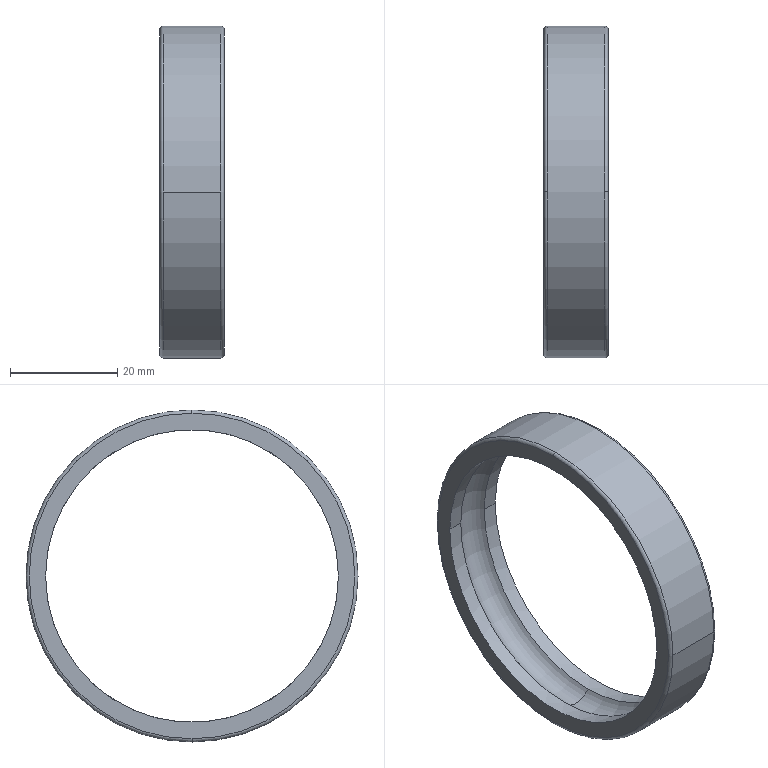Part | STEP file | bearing_6908_02V11 | 1 solid | 14 faces | box 12 x 62 x 62 mm | volume 6668 mm3 | cylinder 6 | torus 6 | plane 2 | commonest cylinder face diameters 54.67 x4 62 x2
STEP:
#1=CARTESIAN_POINT('',(0.,0.,0.));
#2=DIRECTION('',(0.,0.,1.));
#3=DIRECTION('',(1.,0.,0.));
#4=AXIS2_PLACEMENT_3D('',#1,#2,#3);
#5=CARTESIAN_POINT('',(-3.096,27.335,0.));
#6=VERTEX_POINT('',#5);
#7=CARTESIAN_POINT('',(-3.096,0.,27.335));
#8=VERTEX_POINT('',#7);
#9=CARTESIAN_POINT('',(-3.096,0.,0.));
#10=DIRECTION('',(1.,0.,0.));
#11=DIRECTION('',(0.,1.,0.));
#12=AXIS2_PLACEMENT_3D('',#9,#10,#11);
#13=CIRCLE('',#12,27.335);
#14=CARTESIAN_POINT('',(-4.548,0.,0.));
#15=DIRECTION('',(-1.,0.,0.));
#16=DIRECTION('',(0.,1.,0.));
#17=AXIS2_PLACEMENT_3D('',#14,#15,#16);
#18=CYLINDRICAL_SURFACE('',#17,27.335);
#19=CARTESIAN_POINT('',(6.283,-1.452));
#20=DIRECTION('',(-1.,0.));
#21=VECTOR('',#20,1.);
#22=LINE('',#19,#21);
#23=(GEOMETRIC_REPRESENTATION_CONTEXT(2)PARAMETRIC_REPRESENTATION_CONTEXT()REPRESENTATION_CONTEXT('',''));
#24=DEFINITIONAL_REPRESENTATION('',(#22),#23);
#25=PCURVE('',#18,#24);
#26=CARTESIAN_POINT('',(0.,0.,0.));
#27=DIRECTION('',(1.,0.,0.));
#28=DIRECTION('',(0.,0.,-1.));
#29=AXIS2_PLACEMENT_3D('',#26,#27,#28);
#30=TOROIDAL_SURFACE('',#29,25.497,3.6);
#31=CARTESIAN_POINT('',(1.571,-1.035));
#32=DIRECTION('',(1.,0.));
#33=VECTOR('',#32,1.);
#34=LINE('',#31,#33);
#35=(GEOMETRIC_REPRESENTATION_CONTEXT(2)PARAMETRIC_REPRESENTATION_CONTEXT()REPRESENTATION_CONTEXT('',''));
#36=DEFINITIONAL_REPRESENTATION('',(#34),#35);
#37=PCURVE('',#30,#36);
#38=SURFACE_CURVE('',#13,(#25,#37),.PCURVE_S1.);
#39=EDGE_CURVE('',#6,#8,#38,.T.);
#40=ORIENTED_EDGE('',*,*,#39,.F.);
#41=CARTESIAN_POINT('',(-6.,27.335,0.));
#42=VERTEX_POINT('',#41);
#43=CARTESIAN_POINT('',(-4.548,27.335,0.));
#44=DIRECTION('',(-1.,0.,0.));
#45=VECTOR('',#44,1.);
#46=LINE('',#43,#45);
#47=CARTESIAN_POINT('',(6.283,0.));
#48=DIRECTION('',(0.,1.));
#49=VECTOR('',#48,1.);
#50=LINE('',#47,#49);
#51=(GEOMETRIC_REPRESENTATION_CONTEXT(2)PARAMETRIC_REPRESENTATION_CONTEXT()REPRESENTATION_CONTEXT('',''));
#52=DEFINITIONAL_REPRESENTATION('',(#50),#51);
#53=PCURVE('',#18,#52);
#54=CARTESIAN_POINT('',(-4.548,0.,0.));
#55=DIRECTION('',(-1.,0.,0.));
#56=DIRECTION('',(0.,1.,0.));
#57=AXIS2_PLACEMENT_3D('',#54,#55,#56);
#58=CYLINDRICAL_SURFACE('',#57,27.335);
#59=CARTESIAN_POINT('',(0.,0.));
#60=DIRECTION('',(0.,1.));
#61=VECTOR('',#60,1.);
#62=LINE('',#59,#61);
#63=(GEOMETRIC_REPRESENTATION_CONTEXT(2)PARAMETRIC_REPRESENTATION_CONTEXT()REPRESENTATION_CONTEXT('',''));
#64=DEFINITIONAL_REPRESENTATION('',(#62),#63);
#65=PCURVE('',#58,#64);
#66=SURFACE_CURVE('',#46,(#53,#65),.PCURVE_S1.);
#67=EDGE_CURVE('',#6,#42,#66,.T.);
#68=ORIENTED_EDGE('',*,*,#67,.T.);
#69=CARTESIAN_POINT('',(-6.,-27.335,0.));
#70=VERTEX_POINT('',#69);
#71=CARTESIAN_POINT('',(-6.,0.,0.));
#72=DIRECTION('',(1.,0.,0.));
#73=DIRECTION('',(0.,1.,0.));
#74=AXIS2_PLACEMENT_3D('',#71,#72,#73);
#75=CIRCLE('',#74,27.335);
#76=CARTESIAN_POINT('',(6.283,1.452));
#77=DIRECTION('',(-1.,0.));
#78=VECTOR('',#77,1.);
#79=LINE('',#76,#78);
#80=(GEOMETRIC_REPRESENTATION_CONTEXT(2)PARAMETRIC_REPRESENTATION_CONTEXT()REPRESENTATION_CONTEXT('',''));
#81=DEFINITIONAL_REPRESENTATION('',(#79),#80);
#82=PCURVE('',#18,#81);
#83=CARTESIAN_POINT('',(-6.,28.867,0.));
#84=DIRECTION('',(-1.,0.,0.));
#85=DIRECTION('',(0.,-1.,0.));
#86=AXIS2_PLACEMENT_3D('',#83,#84,#85);
#87=PLANE('',#86);
#88=CARTESIAN_POINT('',(1.532,0.));
#89=CARTESIAN_POINT('',(1.532,47.346));
#90=CARTESIAN_POINT('',(42.535,23.673));
#91=CARTESIAN_POINT('',(83.537,0.));
#92=CARTESIAN_POINT('',(42.535,-23.673));
#93=CARTESIAN_POINT('',(1.532,-47.346));
#94=CARTESIAN_POINT('',(1.532,0.));
#95=(BOUNDED_CURVE()B_SPLINE_CURVE(2,(#88,#89,#90,#91,#92,#93,#94),.UNSPECIFIED.,.T.,.F.)B_SPLINE_CURVE_WITH_KNOTS((1,2,2,2,2,1),(-2.094,0.,2.094,4.189,6.283,8.378),.UNSPECIFIED.)CURVE()GEOMETRIC_REPRESENTATION_ITEM()RATIONAL_B_SPLINE_CURVE((1.,0.5,1.,0.5,1.,0.5,1.))REPRESENTATION_ITEM(''));
#96=(GEOMETRIC_REPRESENTATION_CONTEXT(2)PARAMETRIC_REPRESENTATION_CONTEXT()REPRESENTATION_CONTEXT('',''));
#97=DEFINITIONAL_REPRESENTATION('',(#95),#96);
#98=PCURVE('',#87,#97);
#99=SURFACE_CURVE('',#75,(#82,#98),.PCURVE_S1.);
#100=EDGE_CURVE('',#42,#70,#99,.T.);
#101=ORIENTED_EDGE('',*,*,#100,.T.);
#102=CARTESIAN_POINT('',(-3.096,-27.335,0.));
#103=VERTEX_POINT('',#102);
#104=CARTESIAN_POINT('',(-4.548,-27.335,0.));
#105=DIRECTION('',(-1.,0.,0.));
#106=VECTOR('',#105,1.);
#107=LINE('',#104,#106);
#108=CARTESIAN_POINT('',(3.142,0.));
#109=DIRECTION('',(0.,1.));
#110=VECTOR('',#109,1.);
#111=LINE('',#108,#110);
#112=(GEOMETRIC_REPRESENTATION_CONTEXT(2)PARAMETRIC_REPRESENTATION_CONTEXT()REPRESENTATION_CONTEXT('',''));
#113=DEFINITIONAL_REPRESENTATION('',(#111),#112);
#114=PCURVE('',#18,#113);
#115=CARTESIAN_POINT('',(3.142,0.));
#116=DIRECTION('',(0.,1.));
#117=VECTOR('',#116,1.);
#118=LINE('',#115,#117);
#119=(GEOMETRIC_REPRESENTATION_CONTEXT(2)PARAMETRIC_REPRESENTATION_CONTEXT()REPRESENTATION_CONTEXT('',''));
#120=DEFINITIONAL_REPRESENTATION('',(#118),#119);
#121=PCURVE('',#58,#120);
#122=SURFACE_CURVE('',#107,(#114,#121),.PCURVE_S1.);
#123=EDGE_CURVE('',#103,#70,#122,.T.);
#124=ORIENTED_EDGE('',*,*,#123,.F.);
#125=CARTESIAN_POINT('',(-3.096,0.,0.));
#126=DIRECTION('',(1.,0.,0.));
#127=DIRECTION('',(0.,1.,0.));
#128=AXIS2_PLACEMENT_3D('',#125,#126,#127);
#129=CIRCLE('',#128,27.335);
#130=CARTESIAN_POINT('',(6.283,-1.452));
#131=DIRECTION('',(-1.,0.));
#132=VECTOR('',#131,1.);
#133=LINE('',#130,#132);
#134=(GEOMETRIC_REPRESENTATION_CONTEXT(2)PARAMETRIC_REPRESENTATION_CONTEXT()REPRESENTATION_CONTEXT('',''));
#135=DEFINITIONAL_REPRESENTATION('',(#133),#134);
#136=PCURVE('',#18,#135);
#137=CARTESIAN_POINT('',(0.,0.,0.));
#138=DIRECTION('',(1.,0.,0.));
#139=DIRECTION('',(0.,0.,-1.));
#140=AXIS2_PLACEMENT_3D('',#137,#138,#139);
#141=TOROIDAL_SURFACE('',#140,25.497,3.6);
#142=CARTESIAN_POINT('',(1.571,5.248));
#143=DIRECTION('',(1.,0.));
#144=VECTOR('',#143,1.);
#145=LINE('',#142,#144);
#146=(GEOMETRIC_REPRESENTATION_CONTEXT(2)PARAMETRIC_REPRESENTATION_CONTEXT()REPRESENTATION_CONTEXT('',''));
#147=DEFINITIONAL_REPRESENTATION('',(#145),#146);
#148=PCURVE('',#141,#147);
#149=SURFACE_CURVE('',#129,(#136,#148),.PCURVE_S1.);
#150=EDGE_CURVE('',#8,#103,#149,.T.);
#151=ORIENTED_EDGE('',*,*,#150,.F.);
#152=EDGE_LOOP('',(#40,#68,#101,#124,#151));
#153=FACE_BOUND('',#152,.F.);
#154=ADVANCED_FACE('',(#153),#18,.F.);
#155=CARTESIAN_POINT('',(-6.,0.,-30.4));
#156=VERTEX_POINT('',#155);
#157=CARTESIAN_POINT('',(-6.,0.,30.4));
#158=VERTEX_POINT('',#157);
#159=CARTESIAN_POINT('',(-6.,0.,0.));
#160=DIRECTION('',(1.,0.,0.));
#161=DIRECTION('',(0.,1.,0.));
#162=AXIS2_PLACEMENT_3D('',#159,#160,#161);
#163=CIRCLE('',#162,30.4);
#164=CARTESIAN_POINT('',(-5.4,0.,0.));
#165=DIRECTION('',(1.,0.,0.));
#166=DIRECTION('',(0.,0.,-1.));
#167=AXIS2_PLACEMENT_3D('',#164,#165,#166);
#168=TOROIDAL_SURFACE('',#167,30.4,0.6);
#169=CARTESIAN_POINT('',(-4.712,4.712));
#170=DIRECTION('',(1.,0.));
#171=VECTOR('',#170,1.);
#172=LINE('',#169,#171);
#173=(GEOMETRIC_REPRESENTATION_CONTEXT(2)PARAMETRIC_REPRESENTATION_CONTEXT()REPRESENTATION_CONTEXT('',''));
#174=DEFINITIONAL_REPRESENTATION('',(#172),#173);
#175=PCURVE('',#168,#174);
#176=CARTESIAN_POINT('',(-1.532,0.));
#177=CARTESIAN_POINT('',(-1.532,52.654));
#178=CARTESIAN_POINT('',(44.068,26.327));
#179=CARTESIAN_POINT('',(89.668,0.));
#180=CARTESIAN_POINT('',(44.068,-26.327));
#181=CARTESIAN_POINT('',(-1.532,-52.654));
#182=CARTESIAN_POINT('',(-1.532,0.));
#183=(BOUNDED_CURVE()B_SPLINE_CURVE(2,(#176,#177,#178,#179,#180,#181,#182),.UNSPECIFIED.,.T.,.F.)B_SPLINE_CURVE_WITH_KNOTS((1,2,2,2,2,1),(-2.094,0.,2.094,4.189,6.283,8.378),.UNSPECIFIED.)CURVE()GEOMETRIC_REPRESENTATION_ITEM()RATIONAL_B_SPLINE_CURVE((1.,0.5,1.,0.5,1.,0.5,1.))REPRESENTATION_ITEM(''));
#184=(GEOMETRIC_REPRESENTATION_CONTEXT(2)PARAMETRIC_REPRESENTATION_CONTEXT()REPRESENTATION_CONTEXT('',''));
#185=DEFINITIONAL_REPRESENTATION('',(#183),#184);
#186=PCURVE('',#87,#185);
#187=SURFACE_CURVE('',#163,(#175,#186),.PCURVE_S1.);
#188=EDGE_CURVE('',#156,#158,#187,.T.);
#189=ORIENTED_EDGE('',*,*,#188,.T.);
#190=CARTESIAN_POINT('',(-5.4,0.,31.));
#191=VERTEX_POINT('',#190);
#192=CARTESIAN_POINT('',(-5.4,0.,30.4));
#193=DIRECTION('',(0.,1.,0.));
#194=DIRECTION('',(0.,0.,1.));
#195=AXIS2_PLACEMENT_3D('',#192,#193,#194);
#196=CIRCLE('',#195,0.6);
#197=CARTESIAN_POINT('',(3.142,0.));
#198=DIRECTION('',(0.,1.));
#199=VECTOR('',#198,1.);
#200=LINE('',#197,#199);
#201=(GEOMETRIC_REPRESENTATION_CONTEXT(2)PARAMETRIC_REPRESENTATION_CONTEXT()REPRESENTATION_CONTEXT('',''));
#202=DEFINITIONAL_REPRESENTATION('',(#200),#201);
#203=PCURVE('',#168,#202);
#204=CARTESIAN_POINT('',(-5.4,0.,0.));
#205=DIRECTION('',(1.,0.,0.));
#206=DIRECTION('',(0.,0.,-1.));
#207=AXIS2_PLACEMENT_3D('',#204,#205,#206);
#208=TOROIDAL_SURFACE('',#207,30.4,0.6);
#209=CARTESIAN_POINT('',(3.142,0.));
#210=DIRECTION('',(0.,1.));
#211=VECTOR('',#210,1.);
#212=LINE('',#209,#211);
#213=(GEOMETRIC_REPRESENTATION_CONTEXT(2)PARAMETRIC_REPRESENTATION_CONTEXT()REPRESENTATION_CONTEXT('',''));
#214=DEFINITIONAL_REPRESENTATION('',(#212),#213);
#215=PCURVE('',#208,#214);
#216=SURFACE_CURVE('',#196,(#203,#215),.PCURVE_S1.);
#217=EDGE_CURVE('',#158,#191,#216,.T.);
#218=ORIENTED_EDGE('',*,*,#217,.T.);
#219=CARTESIAN_POINT('',(-5.4,31.,0.));
#220=VERTEX_POINT('',#219);
#221=CARTESIAN_POINT('',(-5.4,0.,0.));
#222=DIRECTION('',(1.,0.,0.));
#223=DIRECTION('',(0.,1.,0.));
#224=AXIS2_PLACEMENT_3D('',#221,#222,#223);
#225=CIRCLE('',#224,31.);
#226=CARTESIAN_POINT('',(1.571,6.283));
#227=DIRECTION('',(1.,0.));
#228=VECTOR('',#227,1.);
#229=LINE('',#226,#228);
#230=(GEOMETRIC_REPRESENTATION_CONTEXT(2)PARAMETRIC_REPRESENTATION_CONTEXT()REPRESENTATION_CONTEXT('',''));
#231=DEFINITIONAL_REPRESENTATION('',(#229),#230);
#232=PCURVE('',#168,#231);
#233=CARTESIAN_POINT('',(0.,0.,0.));
#234=DIRECTION('',(-1.,0.,0.));
#235=DIRECTION('',(0.,1.,0.));
#236=AXIS2_PLACEMENT_3D('',#233,#234,#235);
#237=CYLINDRICAL_SURFACE('',#236,31.);
#238=CARTESIAN_POINT('',(6.283,5.4));
#239=DIRECTION('',(-1.,0.));
#240=VECTOR('',#239,1.);
#241=LINE('',#238,#240);
#242=(GEOMETRIC_REPRESENTATION_CONTEXT(2)PARAMETRIC_REPRESENTATION_CONTEXT()REPRESENTATION_CONTEXT('',''));
#243=DEFINITIONAL_REPRESENTATION('',(#241),#242);
#244=PCURVE('',#237,#243);
#245=SURFACE_CURVE('',#225,(#232,#244),.PCURVE_S1.);
#246=EDGE_CURVE('',#220,#191,#245,.T.);
#247=ORIENTED_EDGE('',*,*,#246,.F.);
#248=CARTESIAN_POINT('',(-5.4,0.,-31.));
#249=VERTEX_POINT('',#248);
#250=CARTESIAN_POINT('',(-5.4,0.,0.));
#251=DIRECTION('',(1.,0.,0.));
#252=DIRECTION('',(0.,1.,0.));
#253=AXIS2_PLACEMENT_3D('',#250,#251,#252);
#254=CIRCLE('',#253,31.);
#255=CARTESIAN_POINT('',(-4.712,6.283));
#256=DIRECTION('',(1.,0.));
#257=VECTOR('',#256,1.);
#258=LINE('',#255,#257);
#259=(GEOMETRIC_REPRESENTATION_CONTEXT(2)PARAMETRIC_REPRESENTATION_CONTEXT()REPRESENTATION_CONTEXT('',''));
#260=DEFINITIONAL_REPRESENTATION('',(#258),#259);
#261=PCURVE('',#168,#260);
#262=CARTESIAN_POINT('',(0.,0.,0.));
#263=DIRECTION('',(-1.,0.,0.));
#264=DIRECTION('',(0.,1.,0.));
#265=AXIS2_PLACEMENT_3D('',#262,#263,#264);
#266=CYLINDRICAL_SURFACE('',#265,31.);
#267=CARTESIAN_POINT('',(6.283,5.4));
#268=DIRECTION('',(-1.,0.));
#269=VECTOR('',#268,1.);
#270=LINE('',#267,#269);
#271=(GEOMETRIC_REPRESENTATION_CONTEXT(2)PARAMETRIC_REPRESENTATION_CONTEXT()REPRESENTATION_CONTEXT('',''));
#272=DEFINITIONAL_REPRESENTATION('',(#270),#271);
#273=PCURVE('',#266,#272);
#274=SURFACE_CURVE('',#254,(#261,#273),.PCURVE_S1.);
#275=EDGE_CURVE('',#249,#220,#274,.T.);
#276=ORIENTED_EDGE('',*,*,#275,.F.);
#277=CARTESIAN_POINT('',(-5.4,0.,-30.4));
#278=DIRECTION('',(0.,-1.,0.));
#279=DIRECTION('',(0.,0.,-1.));
#280=AXIS2_PLACEMENT_3D('',#277,#278,#279);
#281=CIRCLE('',#280,0.6);
#282=CARTESIAN_POINT('',(0.,0.));
#283=DIRECTION('',(0.,1.));
#284=VECTOR('',#283,1.);
#285=LINE('',#282,#284);
#286=(GEOMETRIC_REPRESENTATION_CONTEXT(2)PARAMETRIC_REPRESENTATION_CONTEXT()REPRESENTATION_CONTEXT('',''));
#287=DEFINITIONAL_REPRESENTATION('',(#285),#286);
#288=PCURVE('',#168,#287);
#289=CARTESIAN_POINT('',(6.283,0.));
#290=DIRECTION('',(0.,1.));
#291=VECTOR('',#290,1.);
#292=LINE('',#289,#291);
#293=(GEOMETRIC_REPRESENTATION_CONTEXT(2)PARAMETRIC_REPRESENTATION_CONTEXT()REPRESENTATION_CONTEXT('',''));
#294=DEFINITIONAL_REPRESENTATION('',(#292),#293);
#295=PCURVE('',#208,#294);
#296=SURFACE_CURVE('',#281,(#288,#295),.PCURVE_S1.);
#297=EDGE_CURVE('',#156,#249,#296,.T.);
#298=ORIENTED_EDGE('',*,*,#297,.F.);
#299=EDGE_LOOP('',(#189,#218,#247,#276,#298));
#300=FACE_BOUND('',#299,.T.);
#301=ADVANCED_FACE('',(#300),#168,.T.);
#302=CARTESIAN_POINT('',(5.4,-31.,0.));
#303=VERTEX_POINT('',#302);
#304=CARTESIAN_POINT('',(5.4,0.,-31.));
#305=VERTEX_POINT('',#304);
#306=CARTESIAN_POINT('',(5.4,0.,0.));
#307=DIRECTION('',(1.,0.,0.));
#308=DIRECTION('',(0.,1.,0.));
#309=AXIS2_PLACEMENT_3D('',#306,#307,#308);
#310=CIRCLE('',#309,31.);
#311=CARTESIAN_POINT('',(6.283,-5.4));
#312=DIRECTION('',(-1.,0.));
#313=VECTOR('',#312,1.);
#314=LINE('',#311,#313);
#315=(GEOMETRIC_REPRESENTATION_CONTEXT(2)PARAMETRIC_REPRESENTATION_CONTEXT()REPRESENTATION_CONTEXT('',''));
#316=DEFINITIONAL_REPRESENTATION('',(#314),#315);
#317=PCURVE('',#266,#316);
#318=CARTESIAN_POINT('',(5.4,0.,0.));
#319=DIRECTION('',(1.,0.,0.));
#320=DIRECTION('',(0.,0.,-1.));
#321=AXIS2_PLACEMENT_3D('',#318,#319,#320);
#322=TOROIDAL_SURFACE('',#321,30.4,0.6);
#323=CARTESIAN_POINT('',(1.571,0.));
#324=DIRECTION('',(1.,0.));
#325=VECTOR('',#324,1.);
#326=LINE('',#323,#325);
#327=(GEOMETRIC_REPRESENTATION_CONTEXT(2)PARAMETRIC_REPRESENTATION_CONTEXT()REPRESENTATION_CONTEXT('',''));
#328=DEFINITIONAL_REPRESENTATION('',(#326),#327);
#329=PCURVE('',#322,#328);
#330=SURFACE_CURVE('',#310,(#317,#329),.PCURVE_S1.);
#331=EDGE_CURVE('',#303,#305,#330,.T.);
#332=ORIENTED_EDGE('',*,*,#331,.F.);
#333=CARTESIAN_POINT('',(-5.4,-31.,0.));
#334=VERTEX_POINT('',#333);
#335=CARTESIAN_POINT('',(0.,-31.,0.));
#336=DIRECTION('',(-1.,0.,0.));
#337=VECTOR('',#336,1.);
#338=LINE('',#335,#337);
#339=CARTESIAN_POINT('',(3.142,0.));
#340=DIRECTION('',(0.,1.));
#341=VECTOR('',#340,1.);
#342=LINE('',#339,#341);
#343=(GEOMETRIC_REPRESENTATION_CONTEXT(2)PARAMETRIC_REPRESENTATION_CONTEXT()REPRESENTATION_CONTEXT('',''));
#344=DEFINITIONAL_REPRESENTATION('',(#342),#343);
#345=PCURVE('',#266,#344);
#346=CARTESIAN_POINT('',(3.142,0.));
#347=DIRECTION('',(0.,1.));
#348=VECTOR('',#347,1.);
#349=LINE('',#346,#348);
#350=(GEOMETRIC_REPRESENTATION_CONTEXT(2)PARAMETRIC_REPRESENTATION_CONTEXT()REPRESENTATION_CONTEXT('',''));
#351=DEFINITIONAL_REPRESENTATION('',(#349),#350);
#352=PCURVE('',#237,#351);
#353=SURFACE_CURVE('',#338,(#345,#352),.PCURVE_S1.);
#354=EDGE_CURVE('',#303,#334,#353,.T.);
#355=ORIENTED_EDGE('',*,*,#354,.T.);
#356=CARTESIAN_POINT('',(-5.4,0.,0.));
#357=DIRECTION('',(1.,0.,0.));
#358=DIRECTION('',(0.,1.,0.));
#359=AXIS2_PLACEMENT_3D('',#356,#357,#358);
#360=CIRCLE('',#359,31.);
#361=CARTESIAN_POINT('',(6.283,5.4));
#362=DIRECTION('',(-1.,0.));
#363=VECTOR('',#362,1.);
#364=LINE('',#361,#363);
#365=(GEOMETRIC_REPRESENTATION_CONTEXT(2)PARAMETRIC_REPRESENTATION_CONTEXT()REPRESENTATION_CONTEXT('',''));
#366=DEFINITIONAL_REPRESENTATION('',(#364),#365);
#367=PCURVE('',#266,#366);
#368=CARTESIAN_POINT('',(1.571,6.283));
#369=DIRECTION('',(1.,0.));
#370=VECTOR('',#369,1.);
#371=LINE('',#368,#370);
#372=(GEOMETRIC_REPRESENTATION_CONTEXT(2)PARAMETRIC_REPRESENTATION_CONTEXT()REPRESENTATION_CONTEXT('',''));
#373=DEFINITIONAL_REPRESENTATION('',(#371),#372);
#374=PCURVE('',#208,#373);
#375=SURFACE_CURVE('',#360,(#367,#374),.PCURVE_S1.);
#376=EDGE_CURVE('',#334,#249,#375,.T.);
#377=ORIENTED_EDGE('',*,*,#376,.T.);
#378=ORIENTED_EDGE('',*,*,#275,.T.);
#379=CARTESIAN_POINT('',(5.4,31.,0.));
#380=VERTEX_POINT('',#379);
#381=CARTESIAN_POINT('',(0.,31.,0.));
#382=DIRECTION('',(-1.,0.,0.));
#383=VECTOR('',#382,1.);
#384=LINE('',#381,#383);
#385=CARTESIAN_POINT('',(0.,0.));
#386=DIRECTION('',(0.,1.));
#387=VECTOR('',#386,1.);
#388=LINE('',#385,#387);
#389=(GEOMETRIC_REPRESENTATION_CONTEXT(2)PARAMETRIC_REPRESENTATION_CONTEXT()REPRESENTATION_CONTEXT('',''));
#390=DEFINITIONAL_REPRESENTATION('',(#388),#389);
#391=PCURVE('',#266,#390);
#392=CARTESIAN_POINT('',(6.283,0.));
#393=DIRECTION('',(0.,1.));
#394=VECTOR('',#393,1.);
#395=LINE('',#392,#394);
#396=(GEOMETRIC_REPRESENTATION_CONTEXT(2)PARAMETRIC_REPRESENTATION_CONTEXT()REPRESENTATION_CONTEXT('',''));
#397=DEFINITIONAL_REPRESENTATION('',(#395),#396);
#398=PCURVE('',#237,#397);
#399=SURFACE_CURVE('',#384,(#391,#398),.PCURVE_S1.);
#400=EDGE_CURVE('',#380,#220,#399,.T.);
#401=ORIENTED_EDGE('',*,*,#400,.F.);
#402=CARTESIAN_POINT('',(5.4,0.,0.));
#403=DIRECTION('',(1.,0.,0.));
#404=DIRECTION('',(0.,1.,0.));
#405=AXIS2_PLACEMENT_3D('',#402,#403,#404);
#406=CIRCLE('',#405,31.);
#407=CARTESIAN_POINT('',(6.283,-5.4));
#408=DIRECTION('',(-1.,0.));
#409=VECTOR('',#408,1.);
#410=LINE('',#407,#409);
#411=(GEOMETRIC_REPRESENTATION_CONTEXT(2)PARAMETRIC_REPRESENTATION_CONTEXT()REPRESENTATION_CONTEXT('',''));
#412=DEFINITIONAL_REPRESENTATION('',(#410),#411);
#413=PCURVE('',#266,#412);
#414=CARTESIAN_POINT('',(5.4,0.,0.));
#415=DIRECTION('',(1.,0.,0.));
#416=DIRECTION('',(0.,0.,-1.));
#417=AXIS2_PLACEMENT_3D('',#414,#415,#416);
#418=TOROIDAL_SURFACE('',#417,30.4,0.6);
#419=CARTESIAN_POINT('',(-4.712,0.));
#420=DIRECTION('',(1.,0.));
#421=VECTOR('',#420,1.);
#422=LINE('',#419,#421);
#423=(GEOMETRIC_REPRESENTATION_CONTEXT(2)PARAMETRIC_REPRESENTATION_CONTEXT()REPRESENTATION_CONTEXT('',''));
#424=DEFINITIONAL_REPRESENTATION('',(#422),#423);
#425=PCURVE('',#418,#424);
#426=SURFACE_CURVE('',#406,(#413,#425),.PCURVE_S1.);
#427=EDGE_CURVE('',#305,#380,#426,.T.);
#428=ORIENTED_EDGE('',*,*,#427,.F.);
#429=EDGE_LOOP('',(#332,#355,#377,#378,#401,#428));
#430=FACE_BOUND('',#429,.T.);
#431=ADVANCED_FACE('',(#430),#266,.T.);
#432=ORIENTED_EDGE('',*,*,#427,.T.);
#433=CARTESIAN_POINT('',(5.4,0.,31.));
#434=VERTEX_POINT('',#433);
#435=CARTESIAN_POINT('',(5.4,0.,0.));
#436=DIRECTION('',(1.,0.,0.));
#437=DIRECTION('',(0.,1.,0.));
#438=AXIS2_PLACEMENT_3D('',#435,#436,#437);
#439=CIRCLE('',#438,31.);
#440=CARTESIAN_POINT('',(1.571,0.));
#441=DIRECTION('',(1.,0.));
#442=VECTOR('',#441,1.);
#443=LINE('',#440,#442);
#444=(GEOMETRIC_REPRESENTATION_CONTEXT(2)PARAMETRIC_REPRESENTATION_CONTEXT()REPRESENTATION_CONTEXT('',''));
#445=DEFINITIONAL_REPRESENTATION('',(#443),#444);
#446=PCURVE('',#418,#445);
#447=CARTESIAN_POINT('',(6.283,-5.4));
#448=DIRECTION('',(-1.,0.));
#449=VECTOR('',#448,1.);
#450=LINE('',#447,#449);
#451=(GEOMETRIC_REPRESENTATION_CONTEXT(2)PARAMETRIC_REPRESENTATION_CONTEXT()REPRESENTATION_CONTEXT('',''));
#452=DEFINITIONAL_REPRESENTATION('',(#450),#451);
#453=PCURVE('',#237,#452);
#454=SURFACE_CURVE('',#439,(#446,#453),.PCURVE_S1.);
#455=EDGE_CURVE('',#380,#434,#454,.T.);
#456=ORIENTED_EDGE('',*,*,#455,.T.);
#457=CARTESIAN_POINT('',(6.,0.,30.4));
#458=VERTEX_POINT('',#457);
#459=CARTESIAN_POINT('',(5.4,0.,30.4));
#460=DIRECTION('',(0.,1.,0.));
#461=DIRECTION('',(0.,0.,1.));
#462=AXIS2_PLACEMENT_3D('',#459,#460,#461);
#463=CIRCLE('',#462,0.6);
#464=CARTESIAN_POINT('',(3.142,0.));
#465=DIRECTION('',(0.,1.));
#466=VECTOR('',#465,1.);
#467=LINE('',#464,#466);
#468=(GEOMETRIC_REPRESENTATION_CONTEXT(2)PARAMETRIC_REPRESENTATION_CONTEXT()REPRESENTATION_CONTEXT('',''));
#469=DEFINITIONAL_REPRESENTATION('',(#467),#468);
#470=PCURVE('',#418,#469);
#471=CARTESIAN_POINT('',(3.142,0.));
#472=DIRECTION('',(0.,1.));
#473=VECTOR('',#472,1.);
#474=LINE('',#471,#473);
#475=(GEOMETRIC_REPRESENTATION_CONTEXT(2)PARAMETRIC_REPRESENTATION_CONTEXT()REPRESENTATION_CONTEXT('',''));
#476=DEFINITIONAL_REPRESENTATION('',(#474),#475);
#477=PCURVE('',#322,#476);
#478=SURFACE_CURVE('',#463,(#470,#477),.PCURVE_S1.);
#479=EDGE_CURVE('',#434,#458,#478,.T.);
#480=ORIENTED_EDGE('',*,*,#479,.T.);
#481=CARTESIAN_POINT('',(6.,0.,-30.4));
#482=VERTEX_POINT('',#481);
#483=CARTESIAN_POINT('',(6.,0.,0.));
#484=DIRECTION('',(1.,0.,0.));
#485=DIRECTION('',(0.,1.,0.));
#486=AXIS2_PLACEMENT_3D('',#483,#484,#485);
#487=CIRCLE('',#486,30.4);
#488=CARTESIAN_POINT('',(-4.712,1.571));
#489=DIRECTION('',(1.,0.));
#490=VECTOR('',#489,1.);
#491=LINE('',#488,#490);
#492=(GEOMETRIC_REPRESENTATION_CONTEXT(2)PARAMETRIC_REPRESENTATION_CONTEXT()REPRESENTATION_CONTEXT('',''));
#493=DEFINITIONAL_REPRESENTATION('',(#491),#492);
#494=PCURVE('',#418,#493);
#495=CARTESIAN_POINT('',(6.,28.867,0.));
#496=DIRECTION('',(1.,0.,0.));
#497=DIRECTION('',(0.,1.,0.));
#498=AXIS2_PLACEMENT_3D('',#495,#496,#497);
#499=PLANE('',#498);
#500=CARTESIAN_POINT('',(-28.867,0.));
#501=DIRECTION('',(1.,0.));
#502=AXIS2_PLACEMENT_2D('',#500,#501);
#503=CIRCLE('',#502,30.4);
#504=(GEOMETRIC_REPRESENTATION_CONTEXT(2)PARAMETRIC_REPRESENTATION_CONTEXT()REPRESENTATION_CONTEXT('',''));
#505=DEFINITIONAL_REPRESENTATION('',(#503),#504);
#506=PCURVE('',#499,#505);
#507=SURFACE_CURVE('',#487,(#494,#506),.PCURVE_S1.);
#508=EDGE_CURVE('',#482,#458,#507,.T.);
#509=ORIENTED_EDGE('',*,*,#508,.F.);
#510=CARTESIAN_POINT('',(5.4,0.,-30.4));
#511=DIRECTION('',(0.,-1.,0.));
#512=DIRECTION('',(0.,0.,-1.));
#513=AXIS2_PLACEMENT_3D('',#510,#511,#512);
#514=CIRCLE('',#513,0.6);
#515=CARTESIAN_POINT('',(0.,0.));
#516=DIRECTION('',(0.,1.));
#517=VECTOR('',#516,1.);
#518=LINE('',#515,#517);
#519=(GEOMETRIC_REPRESENTATION_CONTEXT(2)PARAMETRIC_REPRESENTATION_CONTEXT()REPRESENTATION_CONTEXT('',''));
#520=DEFINITIONAL_REPRESENTATION('',(#518),#519);
#521=PCURVE('',#418,#520);
#522=CARTESIAN_POINT('',(6.283,0.));
#523=DIRECTION('',(0.,1.));
#524=VECTOR('',#523,1.);
#525=LINE('',#522,#524);
#526=(GEOMETRIC_REPRESENTATION_CONTEXT(2)PARAMETRIC_REPRESENTATION_CONTEXT()REPRESENTATION_CONTEXT('',''));
#527=DEFINITIONAL_REPRESENTATION('',(#525),#526);
#528=PCURVE('',#322,#527);
#529=SURFACE_CURVE('',#514,(#521,#528),.PCURVE_S1.);
#530=EDGE_CURVE('',#305,#482,#529,.T.);
#531=ORIENTED_EDGE('',*,*,#530,.F.);
#532=EDGE_LOOP('',(#432,#456,#480,#509,#531));
#533=FACE_BOUND('',#532,.T.);
#534=ADVANCED_FACE('',(#533),#418,.T.);
#535=CARTESIAN_POINT('',(6.,27.335,0.));
#536=VERTEX_POINT('',#535);
#537=CARTESIAN_POINT('',(3.096,27.335,0.));
#538=VERTEX_POINT('',#537);
#539=CARTESIAN_POINT('',(4.548,27.335,0.));
#540=DIRECTION('',(-1.,0.,0.));
#541=VECTOR('',#540,1.);
#542=LINE('',#539,#541);
#543=CARTESIAN_POINT('',(4.548,0.,0.));
#544=DIRECTION('',(-1.,0.,0.));
#545=DIRECTION('',(0.,1.,0.));
#546=AXIS2_PLACEMENT_3D('',#543,#544,#545);
#547=CYLINDRICAL_SURFACE('',#546,27.335);
#548=CARTESIAN_POINT('',(6.283,0.));
#549=DIRECTION('',(0.,1.));
#550=VECTOR('',#549,1.);
#551=LINE('',#548,#550);
#552=(GEOMETRIC_REPRESENTATION_CONTEXT(2)PARAMETRIC_REPRESENTATION_CONTEXT()REPRESENTATION_CONTEXT('',''));
#553=DEFINITIONAL_REPRESENTATION('',(#551),#552);
#554=PCURVE('',#547,#553);
#555=CARTESIAN_POINT('',(4.548,0.,0.));
#556=DIRECTION('',(-1.,0.,0.));
#557=DIRECTION('',(0.,1.,0.));
#558=AXIS2_PLACEMENT_3D('',#555,#556,#557);
#559=CYLINDRICAL_SURFACE('',#558,27.335);
#560=CARTESIAN_POINT('',(0.,0.));
#561=DIRECTION('',(0.,1.));
#562=VECTOR('',#561,1.);
#563=LINE('',#560,#562);
#564=(GEOMETRIC_REPRESENTATION_CONTEXT(2)PARAMETRIC_REPRESENTATION_CONTEXT()REPRESENTATION_CONTEXT('',''));
#565=DEFINITIONAL_REPRESENTATION('',(#563),#564);
#566=PCURVE('',#559,#565);
#567=SURFACE_CURVE('',#542,(#554,#566),.PCURVE_S1.);
#568=EDGE_CURVE('',#536,#538,#567,.T.);
#569=ORIENTED_EDGE('',*,*,#568,.T.);
#570=CARTESIAN_POINT('',(3.096,0.,27.335));
#571=VERTEX_POINT('',#570);
#572=CARTESIAN_POINT('',(3.096,0.,0.));
#573=DIRECTION('',(1.,0.,0.));
#574=DIRECTION('',(0.,1.,0.));
#575=AXIS2_PLACEMENT_3D('',#572,#573,#574);
#576=CIRCLE('',#575,27.335);
#577=CARTESIAN_POINT('',(6.283,1.452));
#578=DIRECTION('',(-1.,0.));
#579=VECTOR('',#578,1.);
#580=LINE('',#577,#579);
#581=(GEOMETRIC_REPRESENTATION_CONTEXT(2)PARAMETRIC_REPRESENTATION_CONTEXT()REPRESENTATION_CONTEXT('',''));
#582=DEFINITIONAL_REPRESENTATION('',(#580),#581);
#583=PCURVE('',#547,#582);
#584=CARTESIAN_POINT('',(1.571,1.035));
#585=DIRECTION('',(1.,0.));
#586=VECTOR('',#585,1.);
#587=LINE('',#584,#586);
#588=(GEOMETRIC_REPRESENTATION_CONTEXT(2)PARAMETRIC_REPRESENTATION_CONTEXT()REPRESENTATION_CONTEXT('',''));
#589=DEFINITIONAL_REPRESENTATION('',(#587),#588);
#590=PCURVE('',#30,#589);
#591=SURFACE_CURVE('',#576,(#583,#590),.PCURVE_S1.);
#592=EDGE_CURVE('',#538,#571,#591,.T.);
#593=ORIENTED_EDGE('',*,*,#592,.T.);
#594=CARTESIAN_POINT('',(3.096,-27.335,0.));
#595=VERTEX_POINT('',#594);
#596=CARTESIAN_POINT('',(3.096,0.,0.));
#597=DIRECTION('',(1.,0.,0.));
#598=DIRECTION('',(0.,1.,0.));
#599=AXIS2_PLACEMENT_3D('',#596,#597,#598);
#600=CIRCLE('',#599,27.335);
#601=CARTESIAN_POINT('',(6.283,1.452));
#602=DIRECTION('',(-1.,0.));
#603=VECTOR('',#602,1.);
#604=LINE('',#601,#603);
#605=(GEOMETRIC_REPRESENTATION_CONTEXT(2)PARAMETRIC_REPRESENTATION_CONTEXT()REPRESENTATION_CONTEXT('',''));
#606=DEFINITIONAL_REPRESENTATION('',(#604),#605);
#607=PCURVE('',#547,#606);
#608=CARTESIAN_POINT('',(1.571,7.318));
#609=DIRECTION('',(1.,0.));
#610=VECTOR('',#609,1.);
#611=LINE('',#608,#610);
#612=(GEOMETRIC_REPRESENTATION_CONTEXT(2)PARAMETRIC_REPRESENTATION_CONTEXT()REPRESENTATION_CONTEXT('',''));
#613=DEFINITIONAL_REPRESENTATION('',(#611),#612);
#614=PCURVE('',#141,#613);
#615=SURFACE_CURVE('',#600,(#607,#614),.PCURVE_S1.);
#616=EDGE_CURVE('',#571,#595,#615,.T.);
#617=ORIENTED_EDGE('',*,*,#616,.T.);
#618=CARTESIAN_POINT('',(6.,-27.335,0.));
#619=VERTEX_POINT('',#618);
#620=CARTESIAN_POINT('',(4.548,-27.335,0.));
#621=DIRECTION('',(-1.,0.,0.));
#622=VECTOR('',#621,1.);
#623=LINE('',#620,#622);
#624=CARTESIAN_POINT('',(3.142,0.));
#625=DIRECTION('',(0.,1.));
#626=VECTOR('',#625,1.);
#627=LINE('',#624,#626);
#628=(GEOMETRIC_REPRESENTATION_CONTEXT(2)PARAMETRIC_REPRESENTATION_CONTEXT()REPRESENTATION_CONTEXT('',''));
#629=DEFINITIONAL_REPRESENTATION('',(#627),#628);
#630=PCURVE('',#547,#629);
#631=CARTESIAN_POINT('',(3.142,0.));
#632=DIRECTION('',(0.,1.));
#633=VECTOR('',#632,1.);
#634=LINE('',#631,#633);
#635=(GEOMETRIC_REPRESENTATION_CONTEXT(2)PARAMETRIC_REPRESENTATION_CONTEXT()REPRESENTATION_CONTEXT('',''));
#636=DEFINITIONAL_REPRESENTATION('',(#634),#635);
#637=PCURVE('',#559,#636);
#638=SURFACE_CURVE('',#623,(#630,#637),.PCURVE_S1.);
#639=EDGE_CURVE('',#619,#595,#638,.T.);
#640=ORIENTED_EDGE('',*,*,#639,.F.);
#641=CARTESIAN_POINT('',(6.,0.,0.));
#642=DIRECTION('',(1.,0.,0.));
#643=DIRECTION('',(0.,1.,0.));
#644=AXIS2_PLACEMENT_3D('',#641,#642,#643);
#645=CIRCLE('',#644,27.335);
#646=CARTESIAN_POINT('',(6.283,-1.452));
#647=DIRECTION('',(-1.,0.));
#648=VECTOR('',#647,1.);
#649=LINE('',#646,#648);
#650=(GEOMETRIC_REPRESENTATION_CONTEXT(2)PARAMETRIC_REPRESENTATION_CONTEXT()REPRESENTATION_CONTEXT('',''));
#651=DEFINITIONAL_REPRESENTATION('',(#649),#650);
#652=PCURVE('',#547,#651);
#653=CARTESIAN_POINT('',(-28.867,0.));
#654=DIRECTION('',(1.,0.));
#655=AXIS2_PLACEMENT_2D('',#653,#654);
#656=CIRCLE('',#655,27.335);
#657=(GEOMETRIC_REPRESENTATION_CONTEXT(2)PARAMETRIC_REPRESENTATION_CONTEXT()REPRESENTATION_CONTEXT('',''));
#658=DEFINITIONAL_REPRESENTATION('',(#656),#657);
#659=PCURVE('',#499,#658);
#660=SURFACE_CURVE('',#645,(#652,#659),.PCURVE_S1.);
#661=EDGE_CURVE('',#536,#619,#660,.T.);
#662=ORIENTED_EDGE('',*,*,#661,.F.);
#663=EDGE_LOOP('',(#569,#593,#617,#640,#662));
#664=FACE_BOUND('',#663,.F.);
#665=ADVANCED_FACE('',(#664),#547,.F.);
#666=CARTESIAN_POINT('',(-3.096,0.,-27.335));
#667=VERTEX_POINT('',#666);
#668=CARTESIAN_POINT('',(-3.096,0.,0.));
#669=DIRECTION('',(1.,0.,0.));
#670=DIRECTION('',(0.,1.,0.));
#671=AXIS2_PLACEMENT_3D('',#668,#669,#670);
#672=CIRCLE('',#671,27.335);
#673=CARTESIAN_POINT('',(1.571,5.248));
#674=DIRECTION('',(1.,0.));
#675=VECTOR('',#674,1.);
#676=LINE('',#673,#675);
#677=(GEOMETRIC_REPRESENTATION_CONTEXT(2)PARAMETRIC_REPRESENTATION_CONTEXT()REPRESENTATION_CONTEXT('',''));
#678=DEFINITIONAL_REPRESENTATION('',(#676),#677);
#679=PCURVE('',#141,#678);
#680=CARTESIAN_POINT('',(6.283,-1.452));
#681=DIRECTION('',(-1.,0.));
#682=VECTOR('',#681,1.);
#683=LINE('',#680,#682);
#684=(GEOMETRIC_REPRESENTATION_CONTEXT(2)PARAMETRIC_REPRESENTATION_CONTEXT()REPRESENTATION_CONTEXT('',''));
#685=DEFINITIONAL_REPRESENTATION('',(#683),#684);
#686=PCURVE('',#58,#685);
#687=SURFACE_CURVE('',#672,(#679,#686),.PCURVE_S1.);
#688=EDGE_CURVE('',#103,#667,#687,.T.);
#689=ORIENTED_EDGE('',*,*,#688,.T.);
#690=CARTESIAN_POINT('',(3.096,0.,-27.335));
#691=VERTEX_POINT('',#690);
#692=CARTESIAN_POINT('',(0.,0.,-25.497));
#693=DIRECTION('',(0.,-1.,0.));
#694=DIRECTION('',(0.,0.,-1.));
#695=AXIS2_PLACEMENT_3D('',#692,#693,#694);
#696=CIRCLE('',#695,3.6);
#697=CARTESIAN_POINT('',(6.283,0.));
#698=DIRECTION('',(0.,1.));
#699=VECTOR('',#698,1.);
#700=LINE('',#697,#699);
#701=(GEOMETRIC_REPRESENTATION_CONTEXT(2)PARAMETRIC_REPRESENTATION_CONTEXT()REPRESENTATION_CONTEXT('',''));
#702=DEFINITIONAL_REPRESENTATION('',(#700),#701);
#703=PCURVE('',#141,#702);
#704=CARTESIAN_POINT('',(0.,-6.283));
#705=DIRECTION('',(0.,1.));
#706=VECTOR('',#705,1.);
#707=LINE('',#704,#706);
#708=(GEOMETRIC_REPRESENTATION_CONTEXT(2)PARAMETRIC_REPRESENTATION_CONTEXT()REPRESENTATION_CONTEXT('',''));
#709=DEFINITIONAL_REPRESENTATION('',(#707),#708);
#710=PCURVE('',#30,#709);
#711=SURFACE_CURVE('',#696,(#703,#710),.PCURVE_S1.);
#712=EDGE_CURVE('',#667,#691,#711,.T.);
#713=ORIENTED_EDGE('',*,*,#712,.T.);
#714=CARTESIAN_POINT('',(3.096,0.,0.));
#715=DIRECTION('',(1.,0.,0.));
#716=DIRECTION('',(0.,1.,0.));
#717=AXIS2_PLACEMENT_3D('',#714,#715,#716);
#718=CIRCLE('',#717,27.335);
#719=CARTESIAN_POINT('',(1.571,7.318));
#720=DIRECTION('',(1.,0.));
#721=VECTOR('',#720,1.);
#722=LINE('',#719,#721);
#723=(GEOMETRIC_REPRESENTATION_CONTEXT(2)PARAMETRIC_REPRESENTATION_CONTEXT()REPRESENTATION_CONTEXT('',''));
#724=DEFINITIONAL_REPRESENTATION('',(#722),#723);
#725=PCURVE('',#141,#724);
#726=CARTESIAN_POINT('',(6.283,1.452));
#727=DIRECTION('',(-1.,0.));
#728=VECTOR('',#727,1.);
#729=LINE('',#726,#728);
#730=(GEOMETRIC_REPRESENTATION_CONTEXT(2)PARAMETRIC_REPRESENTATION_CONTEXT()REPRESENTATION_CONTEXT('',''));
#731=DEFINITIONAL_REPRESENTATION('',(#729),#730);
#732=PCURVE('',#559,#731);
#733=SURFACE_CURVE('',#718,(#725,#732),.PCURVE_S1.);
#734=EDGE_CURVE('',#595,#691,#733,.T.);
#735=ORIENTED_EDGE('',*,*,#734,.F.);
#736=ORIENTED_EDGE('',*,*,#616,.F.);
#737=CARTESIAN_POINT('',(0.,0.,25.497));
#738=DIRECTION('',(0.,1.,0.));
#739=DIRECTION('',(0.,0.,1.));
#740=AXIS2_PLACEMENT_3D('',#737,#738,#739);
#741=CIRCLE('',#740,3.6);
#742=CARTESIAN_POINT('',(3.142,0.));
#743=DIRECTION('',(0.,1.));
#744=VECTOR('',#743,1.);
#745=LINE('',#742,#744);
#746=(GEOMETRIC_REPRESENTATION_CONTEXT(2)PARAMETRIC_REPRESENTATION_CONTEXT()REPRESENTATION_CONTEXT('',''));
#747=DEFINITIONAL_REPRESENTATION('',(#745),#746);
#748=PCURVE('',#141,#747);
#749=CARTESIAN_POINT('',(3.142,-6.283));
#750=DIRECTION('',(0.,1.));
#751=VECTOR('',#750,1.);
#752=LINE('',#749,#751);
#753=(GEOMETRIC_REPRESENTATION_CONTEXT(2)PARAMETRIC_REPRESENTATION_CONTEXT()REPRESENTATION_CONTEXT('',''));
#754=DEFINITIONAL_REPRESENTATION('',(#752),#753);
#755=PCURVE('',#30,#754);
#756=SURFACE_CURVE('',#741,(#748,#755),.PCURVE_S1.);
#757=EDGE_CURVE('',#8,#571,#756,.T.);
#758=ORIENTED_EDGE('',*,*,#757,.F.);
#759=ORIENTED_EDGE('',*,*,#150,.T.);
#760=EDGE_LOOP('',(#689,#713,#735,#736,#758,#759));
#761=FACE_BOUND('',#760,.F.);
#762=ADVANCED_FACE('',(#761),#141,.F.);
#763=ORIENTED_EDGE('',*,*,#592,.F.);
#764=CARTESIAN_POINT('',(3.096,0.,0.));
#765=DIRECTION('',(1.,0.,0.));
#766=DIRECTION('',(0.,1.,0.));
#767=AXIS2_PLACEMENT_3D('',#764,#765,#766);
#768=CIRCLE('',#767,27.335);
#769=CARTESIAN_POINT('',(-4.712,1.035));
#770=DIRECTION('',(1.,0.));
#771=VECTOR('',#770,1.);
#772=LINE('',#769,#771);
#773=(GEOMETRIC_REPRESENTATION_CONTEXT(2)PARAMETRIC_REPRESENTATION_CONTEXT()REPRESENTATION_CONTEXT('',''));
#774=DEFINITIONAL_REPRESENTATION('',(#772),#773);
#775=PCURVE('',#30,#774);
#776=CARTESIAN_POINT('',(6.283,1.452));
#777=DIRECTION('',(-1.,0.));
#778=VECTOR('',#777,1.);
#779=LINE('',#776,#778);
#780=(GEOMETRIC_REPRESENTATION_CONTEXT(2)PARAMETRIC_REPRESENTATION_CONTEXT()REPRESENTATION_CONTEXT('',''));
#781=DEFINITIONAL_REPRESENTATION('',(#779),#780);
#782=PCURVE('',#559,#781);
#783=SURFACE_CURVE('',#768,(#775,#782),.PCURVE_S1.);
#784=EDGE_CURVE('',#691,#538,#783,.T.);
#785=ORIENTED_EDGE('',*,*,#784,.F.);
#786=ORIENTED_EDGE('',*,*,#712,.F.);
#787=CARTESIAN_POINT('',(-3.096,0.,0.));
#788=DIRECTION('',(1.,0.,0.));
#789=DIRECTION('',(0.,1.,0.));
#790=AXIS2_PLACEMENT_3D('',#787,#788,#789);
#791=CIRCLE('',#790,27.335);
#792=CARTESIAN_POINT('',(-4.712,-1.035));
#793=DIRECTION('',(1.,0.));
#794=VECTOR('',#793,1.);
#795=LINE('',#792,#794);
#796=(GEOMETRIC_REPRESENTATION_CONTEXT(2)PARAMETRIC_REPRESENTATION_CONTEXT()REPRESENTATION_CONTEXT('',''));
#797=DEFINITIONAL_REPRESENTATION('',(#795),#796);
#798=PCURVE('',#30,#797);
#799=CARTESIAN_POINT('',(6.283,-1.452));
#800=DIRECTION('',(-1.,0.));
#801=VECTOR('',#800,1.);
#802=LINE('',#799,#801);
#803=(GEOMETRIC_REPRESENTATION_CONTEXT(2)PARAMETRIC_REPRESENTATION_CONTEXT()REPRESENTATION_CONTEXT('',''));
#804=DEFINITIONAL_REPRESENTATION('',(#802),#803);
#805=PCURVE('',#58,#804);
#806=SURFACE_CURVE('',#791,(#798,#805),.PCURVE_S1.);
#807=EDGE_CURVE('',#667,#6,#806,.T.);
#808=ORIENTED_EDGE('',*,*,#807,.T.);
#809=ORIENTED_EDGE('',*,*,#39,.T.);
#810=ORIENTED_EDGE('',*,*,#757,.T.);
#811=EDGE_LOOP('',(#763,#785,#786,#808,#809,#810));
#812=FACE_BOUND('',#811,.F.);
#813=ADVANCED_FACE('',(#812),#30,.F.);
#814=ORIENTED_EDGE('',*,*,#734,.T.);
#815=ORIENTED_EDGE('',*,*,#784,.T.);
#816=ORIENTED_EDGE('',*,*,#568,.F.);
#817=CARTESIAN_POINT('',(6.,0.,0.));
#818=DIRECTION('',(1.,0.,0.));
#819=DIRECTION('',(0.,1.,0.));
#820=AXIS2_PLACEMENT_3D('',#817,#818,#819);
#821=CIRCLE('',#820,27.335);
#822=CARTESIAN_POINT('',(6.283,-1.452));
#823=DIRECTION('',(-1.,0.));
#824=VECTOR('',#823,1.);
#825=LINE('',#822,#824);
#826=(GEOMETRIC_REPRESENTATION_CONTEXT(2)PARAMETRIC_REPRESENTATION_CONTEXT()REPRESENTATION_CONTEXT('',''));
#827=DEFINITIONAL_REPRESENTATION('',(#825),#826);
#828=PCURVE('',#559,#827);
#829=CARTESIAN_POINT('',(-28.867,0.));
#830=DIRECTION('',(1.,0.));
#831=AXIS2_PLACEMENT_2D('',#829,#830);
#832=CIRCLE('',#831,27.335);
#833=(GEOMETRIC_REPRESENTATION_CONTEXT(2)PARAMETRIC_REPRESENTATION_CONTEXT()REPRESENTATION_CONTEXT('',''));
#834=DEFINITIONAL_REPRESENTATION('',(#832),#833);
#835=PCURVE('',#499,#834);
#836=SURFACE_CURVE('',#821,(#828,#835),.PCURVE_S1.);
#837=EDGE_CURVE('',#619,#536,#836,.T.);
#838=ORIENTED_EDGE('',*,*,#837,.F.);
#839=ORIENTED_EDGE('',*,*,#639,.T.);
#840=EDGE_LOOP('',(#814,#815,#816,#838,#839));
#841=FACE_BOUND('',#840,.F.);
#842=ADVANCED_FACE('',(#841),#559,.F.);
#843=ORIENTED_EDGE('',*,*,#508,.T.);
#844=CARTESIAN_POINT('',(6.,0.,0.));
#845=DIRECTION('',(1.,0.,0.));
#846=DIRECTION('',(0.,1.,0.));
#847=AXIS2_PLACEMENT_3D('',#844,#845,#846);
#848=CIRCLE('',#847,30.4);
#849=CARTESIAN_POINT('',(-28.867,0.));
#850=DIRECTION('',(1.,0.));
#851=AXIS2_PLACEMENT_2D('',#849,#850);
#852=CIRCLE('',#851,30.4);
#853=(GEOMETRIC_REPRESENTATION_CONTEXT(2)PARAMETRIC_REPRESENTATION_CONTEXT()REPRESENTATION_CONTEXT('',''));
#854=DEFINITIONAL_REPRESENTATION('',(#852),#853);
#855=PCURVE('',#499,#854);
#856=CARTESIAN_POINT('',(1.571,1.571));
#857=DIRECTION('',(1.,0.));
#858=VECTOR('',#857,1.);
#859=LINE('',#856,#858);
#860=(GEOMETRIC_REPRESENTATION_CONTEXT(2)PARAMETRIC_REPRESENTATION_CONTEXT()REPRESENTATION_CONTEXT('',''));
#861=DEFINITIONAL_REPRESENTATION('',(#859),#860);
#862=PCURVE('',#322,#861);
#863=SURFACE_CURVE('',#848,(#855,#862),.PCURVE_S1.);
#864=EDGE_CURVE('',#458,#482,#863,.T.);
#865=ORIENTED_EDGE('',*,*,#864,.T.);
#866=EDGE_LOOP('',(#843,#865));
#867=FACE_BOUND('',#866,.T.);
#868=ORIENTED_EDGE('',*,*,#661,.F.);
#869=ORIENTED_EDGE('',*,*,#837,.F.);
#870=EDGE_LOOP('',(#868,#869));
#871=FACE_BOUND('',#870,.T.);
#872=ADVANCED_FACE('',(#867,#871),#499,.T.);
#873=ORIENTED_EDGE('',*,*,#479,.F.);
#874=CARTESIAN_POINT('',(5.4,0.,0.));
#875=DIRECTION('',(1.,0.,0.));
#876=DIRECTION('',(0.,1.,0.));
#877=AXIS2_PLACEMENT_3D('',#874,#875,#876);
#878=CIRCLE('',#877,31.);
#879=CARTESIAN_POINT('',(1.571,0.));
#880=DIRECTION('',(1.,0.));
#881=VECTOR('',#880,1.);
#882=LINE('',#879,#881);
#883=(GEOMETRIC_REPRESENTATION_CONTEXT(2)PARAMETRIC_REPRESENTATION_CONTEXT()REPRESENTATION_CONTEXT('',''));
#884=DEFINITIONAL_REPRESENTATION('',(#882),#883);
#885=PCURVE('',#322,#884);
#886=CARTESIAN_POINT('',(6.283,-5.4));
#887=DIRECTION('',(-1.,0.));
#888=VECTOR('',#887,1.);
#889=LINE('',#886,#888);
#890=(GEOMETRIC_REPRESENTATION_CONTEXT(2)PARAMETRIC_REPRESENTATION_CONTEXT()REPRESENTATION_CONTEXT('',''));
#891=DEFINITIONAL_REPRESENTATION('',(#889),#890);
#892=PCURVE('',#237,#891);
#893=SURFACE_CURVE('',#878,(#885,#892),.PCURVE_S1.);
#894=EDGE_CURVE('',#434,#303,#893,.T.);
#895=ORIENTED_EDGE('',*,*,#894,.T.);
#896=ORIENTED_EDGE('',*,*,#331,.T.);
#897=ORIENTED_EDGE('',*,*,#530,.T.);
#898=ORIENTED_EDGE('',*,*,#864,.F.);
#899=EDGE_LOOP('',(#873,#895,#896,#897,#898));
#900=FACE_BOUND('',#899,.T.);
#901=ADVANCED_FACE('',(#900),#322,.T.);
#902=ORIENTED_EDGE('',*,*,#354,.F.);
#903=ORIENTED_EDGE('',*,*,#894,.F.);
#904=ORIENTED_EDGE('',*,*,#455,.F.);
#905=ORIENTED_EDGE('',*,*,#400,.T.);
#906=ORIENTED_EDGE('',*,*,#246,.T.);
#907=CARTESIAN_POINT('',(-5.4,0.,0.));
#908=DIRECTION('',(1.,0.,0.));
#909=DIRECTION('',(0.,1.,0.));
#910=AXIS2_PLACEMENT_3D('',#907,#908,#909);
#911=CIRCLE('',#910,31.);
#912=CARTESIAN_POINT('',(6.283,5.4));
#913=DIRECTION('',(-1.,0.));
#914=VECTOR('',#913,1.);
#915=LINE('',#912,#914);
#916=(GEOMETRIC_REPRESENTATION_CONTEXT(2)PARAMETRIC_REPRESENTATION_CONTEXT()REPRESENTATION_CONTEXT('',''));
#917=DEFINITIONAL_REPRESENTATION('',(#915),#916);
#918=PCURVE('',#237,#917);
#919=CARTESIAN_POINT('',(1.571,6.283));
#920=DIRECTION('',(1.,0.));
#921=VECTOR('',#920,1.);
#922=LINE('',#919,#921);
#923=(GEOMETRIC_REPRESENTATION_CONTEXT(2)PARAMETRIC_REPRESENTATION_CONTEXT()REPRESENTATION_CONTEXT('',''));
#924=DEFINITIONAL_REPRESENTATION('',(#922),#923);
#925=PCURVE('',#208,#924);
#926=SURFACE_CURVE('',#911,(#918,#925),.PCURVE_S1.);
#927=EDGE_CURVE('',#191,#334,#926,.T.);
#928=ORIENTED_EDGE('',*,*,#927,.T.);
#929=EDGE_LOOP('',(#902,#903,#904,#905,#906,#928));
#930=FACE_BOUND('',#929,.T.);
#931=ADVANCED_FACE('',(#930),#237,.T.);
#932=ORIENTED_EDGE('',*,*,#217,.F.);
#933=CARTESIAN_POINT('',(-6.,0.,0.));
#934=DIRECTION('',(1.,0.,0.));
#935=DIRECTION('',(0.,1.,0.));
#936=AXIS2_PLACEMENT_3D('',#933,#934,#935);
#937=CIRCLE('',#936,30.4);
#938=CARTESIAN_POINT('',(1.571,4.712));
#939=DIRECTION('',(1.,0.));
#940=VECTOR('',#939,1.);
#941=LINE('',#938,#940);
#942=(GEOMETRIC_REPRESENTATION_CONTEXT(2)PARAMETRIC_REPRESENTATION_CONTEXT()REPRESENTATION_CONTEXT('',''));
#943=DEFINITIONAL_REPRESENTATION('',(#941),#942);
#944=PCURVE('',#208,#943);
#945=CARTESIAN_POINT('',(-1.532,0.));
#946=CARTESIAN_POINT('',(-1.532,52.654));
#947=CARTESIAN_POINT('',(44.068,26.327));
#948=CARTESIAN_POINT('',(89.668,0.));
#949=CARTESIAN_POINT('',(44.068,-26.327));
#950=CARTESIAN_POINT('',(-1.532,-52.654));
#951=CARTESIAN_POINT('',(-1.532,0.));
#952=(BOUNDED_CURVE()B_SPLINE_CURVE(2,(#945,#946,#947,#948,#949,#950,#951),.UNSPECIFIED.,.T.,.F.)B_SPLINE_CURVE_WITH_KNOTS((1,2,2,2,2,1),(-2.094,0.,2.094,4.189,6.283,8.378),.UNSPECIFIED.)CURVE()GEOMETRIC_REPRESENTATION_ITEM()RATIONAL_B_SPLINE_CURVE((1.,0.5,1.,0.5,1.,0.5,1.))REPRESENTATION_ITEM(''));
#953=(GEOMETRIC_REPRESENTATION_CONTEXT(2)PARAMETRIC_REPRESENTATION_CONTEXT()REPRESENTATION_CONTEXT('',''));
#954=DEFINITIONAL_REPRESENTATION('',(#952),#953);
#955=PCURVE('',#87,#954);
#956=SURFACE_CURVE('',#937,(#944,#955),.PCURVE_S1.);
#957=EDGE_CURVE('',#158,#156,#956,.T.);
#958=ORIENTED_EDGE('',*,*,#957,.T.);
#959=ORIENTED_EDGE('',*,*,#297,.T.);
#960=ORIENTED_EDGE('',*,*,#376,.F.);
#961=ORIENTED_EDGE('',*,*,#927,.F.);
#962=EDGE_LOOP('',(#932,#958,#959,#960,#961));
#963=FACE_BOUND('',#962,.T.);
#964=ADVANCED_FACE('',(#963),#208,.T.);
#965=ORIENTED_EDGE('',*,*,#100,.T.);
#966=CARTESIAN_POINT('',(-6.,0.,0.));
#967=DIRECTION('',(1.,0.,0.));
#968=DIRECTION('',(0.,1.,0.));
#969=AXIS2_PLACEMENT_3D('',#966,#967,#968);
#970=CIRCLE('',#969,27.335);
#971=CARTESIAN_POINT('',(1.532,0.));
#972=CARTESIAN_POINT('',(1.532,47.346));
#973=CARTESIAN_POINT('',(42.535,23.673));
#974=CARTESIAN_POINT('',(83.537,0.));
#975=CARTESIAN_POINT('',(42.535,-23.673));
#976=CARTESIAN_POINT('',(1.532,-47.346));
#977=CARTESIAN_POINT('',(1.532,0.));
#978=(BOUNDED_CURVE()B_SPLINE_CURVE(2,(#971,#972,#973,#974,#975,#976,#977),.UNSPECIFIED.,.T.,.F.)B_SPLINE_CURVE_WITH_KNOTS((1,2,2,2,2,1),(-2.094,0.,2.094,4.189,6.283,8.378),.UNSPECIFIED.)CURVE()GEOMETRIC_REPRESENTATION_ITEM()RATIONAL_B_SPLINE_CURVE((1.,0.5,1.,0.5,1.,0.5,1.))REPRESENTATION_ITEM(''));
#979=(GEOMETRIC_REPRESENTATION_CONTEXT(2)PARAMETRIC_REPRESENTATION_CONTEXT()REPRESENTATION_CONTEXT('',''));
#980=DEFINITIONAL_REPRESENTATION('',(#978),#979);
#981=PCURVE('',#87,#980);
#982=CARTESIAN_POINT('',(6.283,1.452));
#983=DIRECTION('',(-1.,0.));
#984=VECTOR('',#983,1.);
#985=LINE('',#982,#984);
#986=(GEOMETRIC_REPRESENTATION_CONTEXT(2)PARAMETRIC_REPRESENTATION_CONTEXT()REPRESENTATION_CONTEXT('',''));
#987=DEFINITIONAL_REPRESENTATION('',(#985),#986);
#988=PCURVE('',#58,#987);
#989=SURFACE_CURVE('',#970,(#981,#988),.PCURVE_S1.);
#990=EDGE_CURVE('',#70,#42,#989,.T.);
#991=ORIENTED_EDGE('',*,*,#990,.T.);
#992=EDGE_LOOP('',(#965,#991));
#993=FACE_BOUND('',#992,.T.);
#994=ORIENTED_EDGE('',*,*,#188,.F.);
#995=ORIENTED_EDGE('',*,*,#957,.F.);
#996=EDGE_LOOP('',(#994,#995));
#997=FACE_BOUND('',#996,.T.);
#998=ADVANCED_FACE('',(#993,#997),#87,.T.);
#999=ORIENTED_EDGE('',*,*,#990,.T.);
#1000=ORIENTED_EDGE('',*,*,#67,.F.);
#1001=ORIENTED_EDGE('',*,*,#807,.F.);
#1002=ORIENTED_EDGE('',*,*,#688,.F.);
#1003=ORIENTED_EDGE('',*,*,#123,.T.);
#1004=EDGE_LOOP('',(#999,#1000,#1001,#1002,#1003));
#1005=FACE_BOUND('',#1004,.F.);
#1006=ADVANCED_FACE('',(#1005),#58,.F.);
#1007=CLOSED_SHELL('',(#154,#301,#431,#534,#665,#762,#813,#842,#872,#901,#931,#964,#998,#1006));
#1008=MANIFOLD_SOLID_BREP('',#1007);
#1009=(LENGTH_UNIT()NAMED_UNIT(*)SI_UNIT(.MILLI.,.METRE.));
#1010=UNCERTAINTY_MEASURE_WITH_UNIT(LENGTH_MEASURE(0.0000001),#1009,'','');
#1011=(NAMED_UNIT(*)PLANE_ANGLE_UNIT()SI_UNIT($,.RADIAN.));
#1012=(NAMED_UNIT(*)SI_UNIT($,.STERADIAN.)SOLID_ANGLE_UNIT());
#1013=(GEOMETRIC_REPRESENTATION_CONTEXT(3)GLOBAL_UNCERTAINTY_ASSIGNED_CONTEXT((#1010))GLOBAL_UNIT_ASSIGNED_CONTEXT((#1009,#1011,#1012))REPRESENTATION_CONTEXT('',''));
#1014=ADVANCED_BREP_SHAPE_REPRESENTATION('',(#4,#1008),#1013);